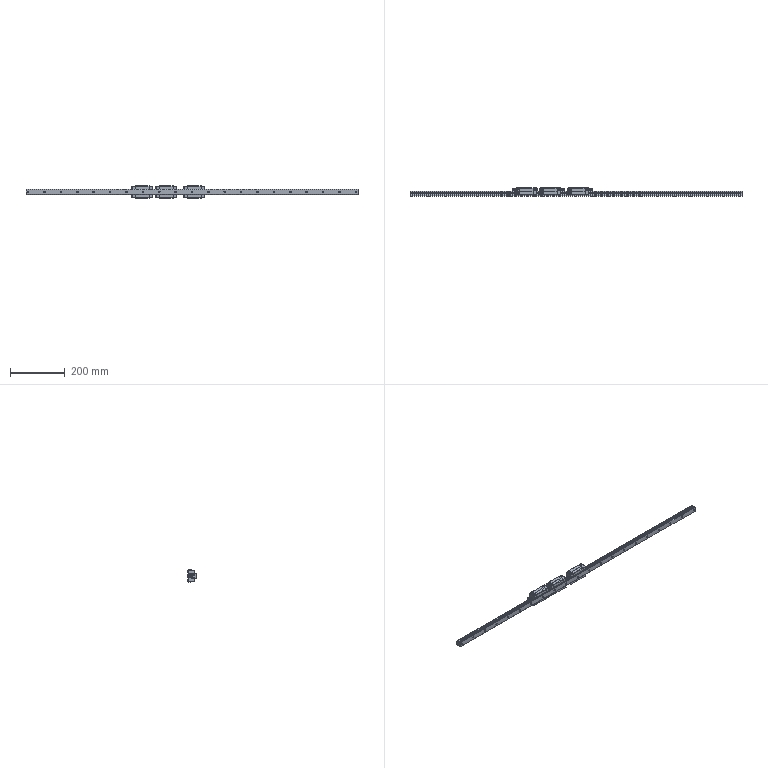Part | SolidWorks | 22 solids | 2431 faces | box 1215 x 30 x 44 mm | volume 550817 mm3 | plane 1496 | cylinder 752 | cone 138 | spline 18 | sphere 18 | torus 9 | commonest cylinder face diameters 1 x216 0.2 x102 2 x88 4.06 x64 0.1 x54 10 x48